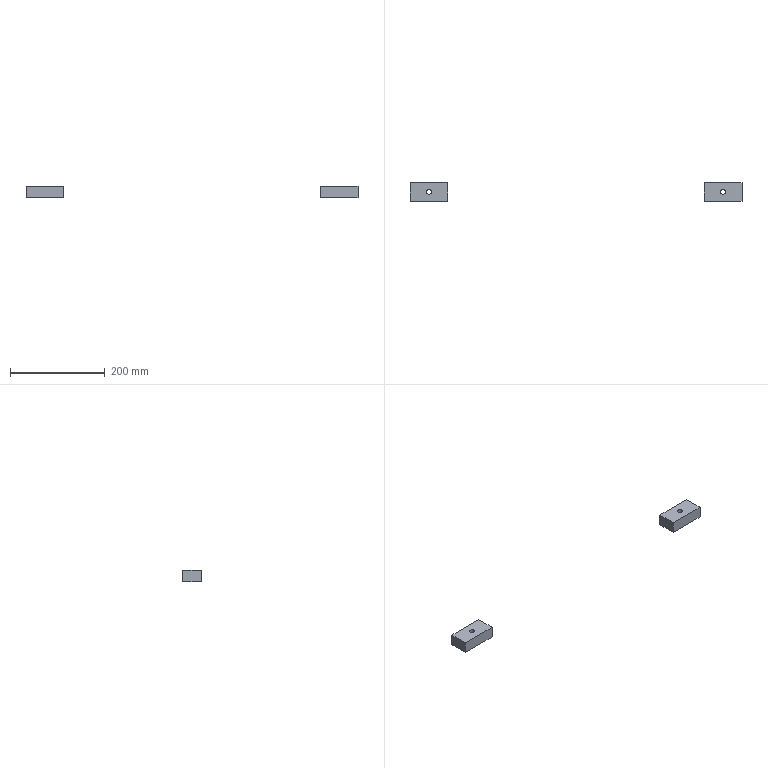Part | SolidWorks | features Extrusion 1, HoleWzd 1 | 2 solids | 16 faces | box 700 x 40 x 25 mm | volume 155914 mm3 | plane 12 | cylinder 4 | commonest cylinder face diameters 10.2 x4
STEP:
#1=CARTESIAN_POINT('',(34.9,-20.,0.));
#2=VERTEX_POINT('',#1);
#3=CARTESIAN_POINT('',(45.1,-20.,0.));
#4=VERTEX_POINT('',#3);
#5=CARTESIAN_POINT('',(40.,-20.,0.));
#6=DIRECTION('',(0.,0.,1.));
#7=DIRECTION('',(1.,0.,0.));
#8=AXIS2_PLACEMENT_3D('',#5,#6,#7);
#9=CIRCLE('',#8,5.1);
#10=EDGE_CURVE('',#2,#4,#9,.T.);
#11=ORIENTED_EDGE('',*,*,#10,.F.);
#12=CARTESIAN_POINT('',(34.9,-20.,25.));
#13=VERTEX_POINT('',#12);
#14=CARTESIAN_POINT('',(34.9,-20.,25.));
#15=DIRECTION('',(0.,0.,1.));
#16=VECTOR('',#15,1000.);
#17=LINE('',#14,#16);
#18=EDGE_CURVE('',#2,#13,#17,.T.);
#19=ORIENTED_EDGE('',*,*,#18,.T.);
#20=CARTESIAN_POINT('',(45.1,-20.,25.));
#21=VERTEX_POINT('',#20);
#22=CARTESIAN_POINT('',(40.,-20.,25.));
#23=DIRECTION('',(0.,0.,1.));
#24=DIRECTION('',(1.,0.,0.));
#25=AXIS2_PLACEMENT_3D('',#22,#23,#24);
#26=CIRCLE('',#25,5.1);
#27=EDGE_CURVE('',#13,#21,#26,.T.);
#28=ORIENTED_EDGE('',*,*,#27,.T.);
#29=CARTESIAN_POINT('',(45.1,-20.,25.));
#30=DIRECTION('',(0.,0.,1.));
#31=VECTOR('',#30,1000.);
#32=LINE('',#29,#31);
#33=EDGE_CURVE('',#4,#21,#32,.T.);
#34=ORIENTED_EDGE('',*,*,#33,.F.);
#35=EDGE_LOOP('',(#11,#19,#28,#34));
#36=FACE_OUTER_BOUND('',#35,.T.);
#37=CARTESIAN_POINT('',(40.,-20.,25.));
#38=DIRECTION('',(0.,0.,1.));
#39=DIRECTION('',(1.,0.,0.));
#40=AXIS2_PLACEMENT_3D('',#37,#38,#39);
#41=CYLINDRICAL_SURFACE('',#40,5.1);
#42=ADVANCED_FACE('',(#36),#41,.F.);
#43=CARTESIAN_POINT('',(0.,0.,0.));
#44=VERTEX_POINT('',#43);
#45=CARTESIAN_POINT('',(0.,-40.,0.));
#46=VERTEX_POINT('',#45);
#47=CARTESIAN_POINT('',(0.,0.,0.));
#48=DIRECTION('',(0.,-1.,0.));
#49=VECTOR('',#48,1000.);
#50=LINE('',#47,#49);
#51=EDGE_CURVE('',#44,#46,#50,.T.);
#52=ORIENTED_EDGE('',*,*,#51,.T.);
#53=CARTESIAN_POINT('',(0.,-40.,25.));
#54=VERTEX_POINT('',#53);
#55=CARTESIAN_POINT('',(0.,-40.,25.));
#56=DIRECTION('',(0.,0.,-1.));
#57=VECTOR('',#56,1000.);
#58=LINE('',#55,#57);
#59=EDGE_CURVE('',#54,#46,#58,.T.);
#60=ORIENTED_EDGE('',*,*,#59,.F.);
#61=CARTESIAN_POINT('',(0.,0.,25.));
#62=VERTEX_POINT('',#61);
#63=CARTESIAN_POINT('',(0.,0.,25.));
#64=DIRECTION('',(0.,-1.,0.));
#65=VECTOR('',#64,1000.);
#66=LINE('',#63,#65);
#67=EDGE_CURVE('',#62,#54,#66,.T.);
#68=ORIENTED_EDGE('',*,*,#67,.F.);
#69=CARTESIAN_POINT('',(0.,0.,25.));
#70=DIRECTION('',(0.,0.,-1.));
#71=VECTOR('',#70,1000.);
#72=LINE('',#69,#71);
#73=EDGE_CURVE('',#62,#44,#72,.T.);
#74=ORIENTED_EDGE('',*,*,#73,.T.);
#75=EDGE_LOOP('',(#52,#60,#68,#74));
#76=FACE_OUTER_BOUND('',#75,.T.);
#77=CARTESIAN_POINT('',(0.,0.,25.));
#78=DIRECTION('',(1.,0.,0.));
#79=DIRECTION('',(0.,0.,-1.));
#80=AXIS2_PLACEMENT_3D('',#77,#78,#79);
#81=PLANE('',#80);
#82=ADVANCED_FACE('',(#76),#81,.F.);
#83=CARTESIAN_POINT('',(80.,-40.,0.));
#84=VERTEX_POINT('',#83);
#85=CARTESIAN_POINT('',(0.,-40.,0.));
#86=DIRECTION('',(1.,0.,0.));
#87=VECTOR('',#86,1000.);
#88=LINE('',#85,#87);
#89=EDGE_CURVE('',#46,#84,#88,.T.);
#90=ORIENTED_EDGE('',*,*,#89,.T.);
#91=CARTESIAN_POINT('',(80.,-40.,25.));
#92=VERTEX_POINT('',#91);
#93=CARTESIAN_POINT('',(80.,-40.,25.));
#94=DIRECTION('',(0.,0.,-1.));
#95=VECTOR('',#94,1000.);
#96=LINE('',#93,#95);
#97=EDGE_CURVE('',#92,#84,#96,.T.);
#98=ORIENTED_EDGE('',*,*,#97,.F.);
#99=CARTESIAN_POINT('',(0.,-40.,25.));
#100=DIRECTION('',(1.,0.,0.));
#101=VECTOR('',#100,1000.);
#102=LINE('',#99,#101);
#103=EDGE_CURVE('',#54,#92,#102,.T.);
#104=ORIENTED_EDGE('',*,*,#103,.F.);
#105=ORIENTED_EDGE('',*,*,#59,.T.);
#106=EDGE_LOOP('',(#90,#98,#104,#105));
#107=FACE_OUTER_BOUND('',#106,.T.);
#108=CARTESIAN_POINT('',(0.,-40.,25.));
#109=DIRECTION('',(0.,1.,0.));
#110=DIRECTION('',(0.,0.,1.));
#111=AXIS2_PLACEMENT_3D('',#108,#109,#110);
#112=PLANE('',#111);
#113=ADVANCED_FACE('',(#107),#112,.F.);
#114=CARTESIAN_POINT('',(80.,0.,0.));
#115=VERTEX_POINT('',#114);
#116=CARTESIAN_POINT('',(80.,0.,0.));
#117=DIRECTION('',(0.,1.,0.));
#118=VECTOR('',#117,1000.);
#119=LINE('',#116,#118);
#120=EDGE_CURVE('',#84,#115,#119,.T.);
#121=ORIENTED_EDGE('',*,*,#120,.T.);
#122=CARTESIAN_POINT('',(80.,0.,25.));
#123=VERTEX_POINT('',#122);
#124=CARTESIAN_POINT('',(80.,0.,25.));
#125=DIRECTION('',(0.,0.,-1.));
#126=VECTOR('',#125,1000.);
#127=LINE('',#124,#126);
#128=EDGE_CURVE('',#123,#115,#127,.T.);
#129=ORIENTED_EDGE('',*,*,#128,.F.);
#130=CARTESIAN_POINT('',(80.,0.,25.));
#131=DIRECTION('',(0.,1.,0.));
#132=VECTOR('',#131,1000.);
#133=LINE('',#130,#132);
#134=EDGE_CURVE('',#92,#123,#133,.T.);
#135=ORIENTED_EDGE('',*,*,#134,.F.);
#136=ORIENTED_EDGE('',*,*,#97,.T.);
#137=EDGE_LOOP('',(#121,#129,#135,#136));
#138=FACE_OUTER_BOUND('',#137,.T.);
#139=CARTESIAN_POINT('',(80.,0.,25.));
#140=DIRECTION('',(-1.,0.,0.));
#141=DIRECTION('',(0.,-1.,0.));
#142=AXIS2_PLACEMENT_3D('',#139,#140,#141);
#143=PLANE('',#142);
#144=ADVANCED_FACE('',(#138),#143,.F.);
#145=CARTESIAN_POINT('',(0.,0.,0.));
#146=DIRECTION('',(-1.,0.,0.));
#147=VECTOR('',#146,1000.);
#148=LINE('',#145,#147);
#149=EDGE_CURVE('',#115,#44,#148,.T.);
#150=ORIENTED_EDGE('',*,*,#149,.T.);
#151=ORIENTED_EDGE('',*,*,#73,.F.);
#152=CARTESIAN_POINT('',(0.,0.,25.));
#153=DIRECTION('',(-1.,0.,0.));
#154=VECTOR('',#153,1000.);
#155=LINE('',#152,#154);
#156=EDGE_CURVE('',#123,#62,#155,.T.);
#157=ORIENTED_EDGE('',*,*,#156,.F.);
#158=ORIENTED_EDGE('',*,*,#128,.T.);
#159=EDGE_LOOP('',(#150,#151,#157,#158));
#160=FACE_OUTER_BOUND('',#159,.T.);
#161=CARTESIAN_POINT('',(0.,0.,25.));
#162=DIRECTION('',(0.,-1.,0.));
#163=DIRECTION('',(0.,0.,-1.));
#164=AXIS2_PLACEMENT_3D('',#161,#162,#163);
#165=PLANE('',#164);
#166=ADVANCED_FACE('',(#160),#165,.F.);
#167=CARTESIAN_POINT('',(40.,-20.,25.));
#168=DIRECTION('',(0.,0.,1.));
#169=DIRECTION('',(1.,0.,0.));
#170=AXIS2_PLACEMENT_3D('',#167,#168,#169);
#171=CIRCLE('',#170,5.1);
#172=EDGE_CURVE('',#21,#13,#171,.T.);
#173=ORIENTED_EDGE('',*,*,#172,.F.);
#174=ORIENTED_EDGE('',*,*,#27,.F.);
#175=EDGE_LOOP('',(#173,#174));
#176=FACE_BOUND('',#175,.T.);
#177=ORIENTED_EDGE('',*,*,#67,.T.);
#178=ORIENTED_EDGE('',*,*,#103,.T.);
#179=ORIENTED_EDGE('',*,*,#134,.T.);
#180=ORIENTED_EDGE('',*,*,#156,.T.);
#181=EDGE_LOOP('',(#177,#178,#179,#180));
#182=FACE_OUTER_BOUND('',#181,.T.);
#183=CARTESIAN_POINT('',(0.,0.,25.));
#184=DIRECTION('',(0.,0.,1.));
#185=DIRECTION('',(1.,0.,0.));
#186=AXIS2_PLACEMENT_3D('',#183,#184,#185);
#187=PLANE('',#186);
#188=ADVANCED_FACE('',(#176,#182),#187,.T.);
#189=CARTESIAN_POINT('',(40.,-20.,0.));
#190=DIRECTION('',(0.,0.,1.));
#191=DIRECTION('',(1.,0.,0.));
#192=AXIS2_PLACEMENT_3D('',#189,#190,#191);
#193=CIRCLE('',#192,5.1);
#194=EDGE_CURVE('',#4,#2,#193,.T.);
#195=ORIENTED_EDGE('',*,*,#194,.T.);
#196=ORIENTED_EDGE('',*,*,#10,.T.);
#197=EDGE_LOOP('',(#195,#196));
#198=FACE_BOUND('',#197,.T.);
#199=ORIENTED_EDGE('',*,*,#51,.F.);
#200=ORIENTED_EDGE('',*,*,#149,.F.);
#201=ORIENTED_EDGE('',*,*,#120,.F.);
#202=ORIENTED_EDGE('',*,*,#89,.F.);
#203=EDGE_LOOP('',(#199,#200,#201,#202));
#204=FACE_OUTER_BOUND('',#203,.T.);
#205=CARTESIAN_POINT('',(0.,0.,0.));
#206=DIRECTION('',(0.,0.,1.));
#207=DIRECTION('',(1.,0.,0.));
#208=AXIS2_PLACEMENT_3D('',#205,#206,#207);
#209=PLANE('',#208);
#210=ADVANCED_FACE('',(#198,#204),#209,.F.);
#211=ORIENTED_EDGE('',*,*,#18,.F.);
#212=ORIENTED_EDGE('',*,*,#194,.F.);
#213=ORIENTED_EDGE('',*,*,#33,.T.);
#214=ORIENTED_EDGE('',*,*,#172,.T.);
#215=EDGE_LOOP('',(#211,#212,#213,#214));
#216=FACE_OUTER_BOUND('',#215,.T.);
#217=CARTESIAN_POINT('',(40.,-20.,25.));
#218=DIRECTION('',(0.,0.,1.));
#219=DIRECTION('',(1.,0.,0.));
#220=AXIS2_PLACEMENT_3D('',#217,#218,#219);
#221=CYLINDRICAL_SURFACE('',#220,5.1);
#222=ADVANCED_FACE('',(#216),#221,.F.);
#223=CLOSED_SHELL('',(#42,#82,#113,#144,#166,#188,#210,#222));
#224=MANIFOLD_SOLID_BREP('',#223);
#225=CARTESIAN_POINT('',(654.9,-20.,0.));
#226=VERTEX_POINT('',#225);
#227=CARTESIAN_POINT('',(665.1,-20.,0.));
#228=VERTEX_POINT('',#227);
#229=CARTESIAN_POINT('',(660.,-20.,0.));
#230=DIRECTION('',(0.,0.,1.));
#231=DIRECTION('',(1.,0.,0.));
#232=AXIS2_PLACEMENT_3D('',#229,#230,#231);
#233=CIRCLE('',#232,5.1);
#234=EDGE_CURVE('',#226,#228,#233,.T.);
#235=ORIENTED_EDGE('',*,*,#234,.F.);
#236=CARTESIAN_POINT('',(654.9,-20.,25.));
#237=VERTEX_POINT('',#236);
#238=CARTESIAN_POINT('',(654.9,-20.,25.));
#239=DIRECTION('',(0.,0.,1.));
#240=VECTOR('',#239,1000.);
#241=LINE('',#238,#240);
#242=EDGE_CURVE('',#226,#237,#241,.T.);
#243=ORIENTED_EDGE('',*,*,#242,.T.);
#244=CARTESIAN_POINT('',(665.1,-20.,25.));
#245=VERTEX_POINT('',#244);
#246=CARTESIAN_POINT('',(660.,-20.,25.));
#247=DIRECTION('',(0.,0.,1.));
#248=DIRECTION('',(1.,0.,0.));
#249=AXIS2_PLACEMENT_3D('',#246,#247,#248);
#250=CIRCLE('',#249,5.1);
#251=EDGE_CURVE('',#237,#245,#250,.T.);
#252=ORIENTED_EDGE('',*,*,#251,.T.);
#253=CARTESIAN_POINT('',(665.1,-20.,25.));
#254=DIRECTION('',(0.,0.,1.));
#255=VECTOR('',#254,1000.);
#256=LINE('',#253,#255);
#257=EDGE_CURVE('',#228,#245,#256,.T.);
#258=ORIENTED_EDGE('',*,*,#257,.F.);
#259=EDGE_LOOP('',(#235,#243,#252,#258));
#260=FACE_OUTER_BOUND('',#259,.T.);
#261=CARTESIAN_POINT('',(660.,-20.,25.));
#262=DIRECTION('',(0.,0.,1.));
#263=DIRECTION('',(1.,0.,0.));
#264=AXIS2_PLACEMENT_3D('',#261,#262,#263);
#265=CYLINDRICAL_SURFACE('',#264,5.1);
#266=ADVANCED_FACE('',(#260),#265,.F.);
#267=CARTESIAN_POINT('',(620.,0.,0.));
#268=VERTEX_POINT('',#267);
#269=CARTESIAN_POINT('',(620.,-40.,0.));
#270=VERTEX_POINT('',#269);
#271=CARTESIAN_POINT('',(620.,0.,0.));
#272=DIRECTION('',(0.,-1.,0.));
#273=VECTOR('',#272,1000.);
#274=LINE('',#271,#273);
#275=EDGE_CURVE('',#268,#270,#274,.T.);
#276=ORIENTED_EDGE('',*,*,#275,.T.);
#277=CARTESIAN_POINT('',(620.,-40.,25.));
#278=VERTEX_POINT('',#277);
#279=CARTESIAN_POINT('',(620.,-40.,25.));
#280=DIRECTION('',(0.,0.,-1.));
#281=VECTOR('',#280,1000.);
#282=LINE('',#279,#281);
#283=EDGE_CURVE('',#278,#270,#282,.T.);
#284=ORIENTED_EDGE('',*,*,#283,.F.);
#285=CARTESIAN_POINT('',(620.,0.,25.));
#286=VERTEX_POINT('',#285);
#287=CARTESIAN_POINT('',(620.,0.,25.));
#288=DIRECTION('',(0.,-1.,0.));
#289=VECTOR('',#288,1000.);
#290=LINE('',#287,#289);
#291=EDGE_CURVE('',#286,#278,#290,.T.);
#292=ORIENTED_EDGE('',*,*,#291,.F.);
#293=CARTESIAN_POINT('',(620.,0.,25.));
#294=DIRECTION('',(0.,0.,-1.));
#295=VECTOR('',#294,1000.);
#296=LINE('',#293,#295);
#297=EDGE_CURVE('',#286,#268,#296,.T.);
#298=ORIENTED_EDGE('',*,*,#297,.T.);
#299=EDGE_LOOP('',(#276,#284,#292,#298));
#300=FACE_OUTER_BOUND('',#299,.T.);
#301=CARTESIAN_POINT('',(620.,0.,25.));
#302=DIRECTION('',(1.,0.,0.));
#303=DIRECTION('',(0.,0.,-1.));
#304=AXIS2_PLACEMENT_3D('',#301,#302,#303);
#305=PLANE('',#304);
#306=ADVANCED_FACE('',(#300),#305,.F.);
#307=CARTESIAN_POINT('',(700.,-40.,0.));
#308=VERTEX_POINT('',#307);
#309=CARTESIAN_POINT('',(620.,-40.,0.));
#310=DIRECTION('',(1.,0.,0.));
#311=VECTOR('',#310,1000.);
#312=LINE('',#309,#311);
#313=EDGE_CURVE('',#270,#308,#312,.T.);
#314=ORIENTED_EDGE('',*,*,#313,.T.);
#315=CARTESIAN_POINT('',(700.,-40.,25.));
#316=VERTEX_POINT('',#315);
#317=CARTESIAN_POINT('',(700.,-40.,25.));
#318=DIRECTION('',(0.,0.,-1.));
#319=VECTOR('',#318,1000.);
#320=LINE('',#317,#319);
#321=EDGE_CURVE('',#316,#308,#320,.T.);
#322=ORIENTED_EDGE('',*,*,#321,.F.);
#323=CARTESIAN_POINT('',(620.,-40.,25.));
#324=DIRECTION('',(1.,0.,0.));
#325=VECTOR('',#324,1000.);
#326=LINE('',#323,#325);
#327=EDGE_CURVE('',#278,#316,#326,.T.);
#328=ORIENTED_EDGE('',*,*,#327,.F.);
#329=ORIENTED_EDGE('',*,*,#283,.T.);
#330=EDGE_LOOP('',(#314,#322,#328,#329));
#331=FACE_OUTER_BOUND('',#330,.T.);
#332=CARTESIAN_POINT('',(620.,-40.,25.));
#333=DIRECTION('',(0.,1.,0.));
#334=DIRECTION('',(0.,0.,1.));
#335=AXIS2_PLACEMENT_3D('',#332,#333,#334);
#336=PLANE('',#335);
#337=ADVANCED_FACE('',(#331),#336,.F.);
#338=CARTESIAN_POINT('',(700.,0.,0.));
#339=VERTEX_POINT('',#338);
#340=CARTESIAN_POINT('',(700.,0.,0.));
#341=DIRECTION('',(0.,1.,0.));
#342=VECTOR('',#341,1000.);
#343=LINE('',#340,#342);
#344=EDGE_CURVE('',#308,#339,#343,.T.);
#345=ORIENTED_EDGE('',*,*,#344,.T.);
#346=CARTESIAN_POINT('',(700.,0.,25.));
#347=VERTEX_POINT('',#346);
#348=CARTESIAN_POINT('',(700.,0.,25.));
#349=DIRECTION('',(0.,0.,-1.));
#350=VECTOR('',#349,1000.);
#351=LINE('',#348,#350);
#352=EDGE_CURVE('',#347,#339,#351,.T.);
#353=ORIENTED_EDGE('',*,*,#352,.F.);
#354=CARTESIAN_POINT('',(700.,0.,25.));
#355=DIRECTION('',(0.,1.,0.));
#356=VECTOR('',#355,1000.);
#357=LINE('',#354,#356);
#358=EDGE_CURVE('',#316,#347,#357,.T.);
#359=ORIENTED_EDGE('',*,*,#358,.F.);
#360=ORIENTED_EDGE('',*,*,#321,.T.);
#361=EDGE_LOOP('',(#345,#353,#359,#360));
#362=FACE_OUTER_BOUND('',#361,.T.);
#363=CARTESIAN_POINT('',(700.,0.,25.));
#364=DIRECTION('',(-1.,0.,0.));
#365=DIRECTION('',(0.,0.,1.));
#366=AXIS2_PLACEMENT_3D('',#363,#364,#365);
#367=PLANE('',#366);
#368=ADVANCED_FACE('',(#362),#367,.F.);
#369=CARTESIAN_POINT('',(620.,0.,0.));
#370=DIRECTION('',(-1.,0.,0.));
#371=VECTOR('',#370,1000.);
#372=LINE('',#369,#371);
#373=EDGE_CURVE('',#339,#268,#372,.T.);
#374=ORIENTED_EDGE('',*,*,#373,.T.);
#375=ORIENTED_EDGE('',*,*,#297,.F.);
#376=CARTESIAN_POINT('',(620.,0.,25.));
#377=DIRECTION('',(-1.,0.,0.));
#378=VECTOR('',#377,1000.);
#379=LINE('',#376,#378);
#380=EDGE_CURVE('',#347,#286,#379,.T.);
#381=ORIENTED_EDGE('',*,*,#380,.F.);
#382=ORIENTED_EDGE('',*,*,#352,.T.);
#383=EDGE_LOOP('',(#374,#375,#381,#382));
#384=FACE_OUTER_BOUND('',#383,.T.);
#385=CARTESIAN_POINT('',(620.,0.,25.));
#386=DIRECTION('',(0.,-1.,0.));
#387=DIRECTION('',(0.,0.,-1.));
#388=AXIS2_PLACEMENT_3D('',#385,#386,#387);
#389=PLANE('',#388);
#390=ADVANCED_FACE('',(#384),#389,.F.);
#391=CARTESIAN_POINT('',(660.,-20.,25.));
#392=DIRECTION('',(0.,0.,1.));
#393=DIRECTION('',(1.,0.,0.));
#394=AXIS2_PLACEMENT_3D('',#391,#392,#393);
#395=CIRCLE('',#394,5.1);
#396=EDGE_CURVE('',#245,#237,#395,.T.);
#397=ORIENTED_EDGE('',*,*,#396,.F.);
#398=ORIENTED_EDGE('',*,*,#251,.F.);
#399=EDGE_LOOP('',(#397,#398));
#400=FACE_BOUND('',#399,.T.);
#401=ORIENTED_EDGE('',*,*,#291,.T.);
#402=ORIENTED_EDGE('',*,*,#327,.T.);
#403=ORIENTED_EDGE('',*,*,#358,.T.);
#404=ORIENTED_EDGE('',*,*,#380,.T.);
#405=EDGE_LOOP('',(#401,#402,#403,#404));
#406=FACE_OUTER_BOUND('',#405,.T.);
#407=CARTESIAN_POINT('',(0.,0.,25.));
#408=DIRECTION('',(0.,0.,1.));
#409=DIRECTION('',(1.,0.,0.));
#410=AXIS2_PLACEMENT_3D('',#407,#408,#409);
#411=PLANE('',#410);
#412=ADVANCED_FACE('',(#400,#406),#411,.T.);
#413=CARTESIAN_POINT('',(660.,-20.,0.));
#414=DIRECTION('',(0.,0.,1.));
#415=DIRECTION('',(1.,0.,0.));
#416=AXIS2_PLACEMENT_3D('',#413,#414,#415);
#417=CIRCLE('',#416,5.1);
#418=EDGE_CURVE('',#228,#226,#417,.T.);
#419=ORIENTED_EDGE('',*,*,#418,.T.);
#420=ORIENTED_EDGE('',*,*,#234,.T.);
#421=EDGE_LOOP('',(#419,#420));
#422=FACE_BOUND('',#421,.T.);
#423=ORIENTED_EDGE('',*,*,#275,.F.);
#424=ORIENTED_EDGE('',*,*,#373,.F.);
#425=ORIENTED_EDGE('',*,*,#344,.F.);
#426=ORIENTED_EDGE('',*,*,#313,.F.);
#427=EDGE_LOOP('',(#423,#424,#425,#426));
#428=FACE_OUTER_BOUND('',#427,.T.);
#429=CARTESIAN_POINT('',(0.,0.,0.));
#430=DIRECTION('',(0.,0.,1.));
#431=DIRECTION('',(1.,0.,0.));
#432=AXIS2_PLACEMENT_3D('',#429,#430,#431);
#433=PLANE('',#432);
#434=ADVANCED_FACE('',(#422,#428),#433,.F.);
#435=ORIENTED_EDGE('',*,*,#242,.F.);
#436=ORIENTED_EDGE('',*,*,#418,.F.);
#437=ORIENTED_EDGE('',*,*,#257,.T.);
#438=ORIENTED_EDGE('',*,*,#396,.T.);
#439=EDGE_LOOP('',(#435,#436,#437,#438));
#440=FACE_OUTER_BOUND('',#439,.T.);
#441=CARTESIAN_POINT('',(660.,-20.,25.));
#442=DIRECTION('',(0.,0.,1.));
#443=DIRECTION('',(1.,0.,0.));
#444=AXIS2_PLACEMENT_3D('',#441,#442,#443);
#445=CYLINDRICAL_SURFACE('',#444,5.1);
#446=ADVANCED_FACE('',(#440),#445,.F.);
#447=CLOSED_SHELL('',(#266,#306,#337,#368,#390,#412,#434,#446));
#448=MANIFOLD_SOLID_BREP('',#447);
#449=CARTESIAN_POINT('',(0.,0.,0.));
#450=DIRECTION('',(0.,0.,1.));
#451=DIRECTION('',(1.,0.,0.));
#452=AXIS2_PLACEMENT_3D('',#449,#450,#451);
#453=(LENGTH_UNIT()NAMED_UNIT(*)SI_UNIT(.MILLI.,.METRE.));
#454=UNCERTAINTY_MEASURE_WITH_UNIT(LENGTH_MEASURE(0.00001),#453,'','');
#455=(NAMED_UNIT(*)PLANE_ANGLE_UNIT()SI_UNIT($,.RADIAN.));
#456=(NAMED_UNIT(*)SI_UNIT($,.STERADIAN.)SOLID_ANGLE_UNIT());
#457=(GEOMETRIC_REPRESENTATION_CONTEXT(3)GLOBAL_UNCERTAINTY_ASSIGNED_CONTEXT((#454))GLOBAL_UNIT_ASSIGNED_CONTEXT((#453,#455,#456))REPRESENTATION_CONTEXT('',''));
#458=ADVANCED_BREP_SHAPE_REPRESENTATION('',(#224,#448,#452),#457);